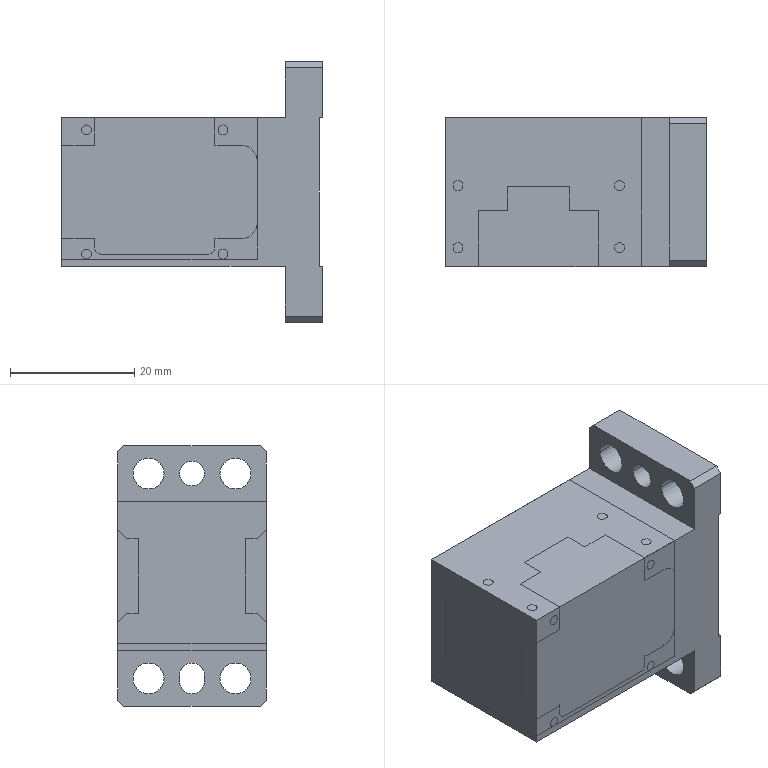NC program | NX | posted with a generic post | part box 42 x 24 x 42 mm
Lines 10409 to 10692 of 10692:
(PLANAR_MILL_COPY_2 , TOOL : D6A45)
N20798 T07 M6
N20800 G54
N20802 G17 G0 G90 X-6.753 Y16.814 B0. C0. S7500 M3
N20804 G43 Z30. H7
N20806 Z0.5
N20808 G94 G1 Z-1. F1250.
N20810 X-6.134 Y17.6
N20812 G3 X-7. Y18.1 R1.
N20814 X-8.6 Y16.5 R1.6
N20816 X-7. Y18.1 R-1.6
N20818 X-7.866 Y17.6 R1.
N20820 G1 X-7.247 Y16.814
N20822 Z0.5
N20824 G0 Z30.
N20826 X-1.063 Y16.825
N20828 Z0.5
N20830 G1 X-1.1 Y16.759 Z0.48
N20832 Y16.5 Z0.41
N20834 Y16.241 Z0.341
N20836 X-0.799 Y15.701 Z0.175
N20838 X-0.259 Y15.4 Z0.009
N20840 X0.259 Z-0.129
N20842 X0.799 Y15.701 Z-0.295
N20844 X1.1 Y16.241 Z-0.461
N20846 Y16.759 Z-0.599
N20848 X0.799 Y17.299 Z-0.765
N20850 X0.259 Y17.6 Z-0.931
N20852 X0. Z-1.
N20854 G3 X-1.1 Y16.5 R1.1
N20856 X0. Y17.6 R-1.1
N20858 X-0.866 Y17.1 R1.
N20860 G1 Z0.5
N20862 G0 Z30.
N20864 X7.247 Y16.814
N20866 Z0.5
N20868 G1 Z-1.
N20870 X7.866 Y17.6
N20872 G3 X7. Y18.1 R1.
N20874 X5.4 Y16.5 R1.6
N20876 X7. Y18.1 R-1.6
N20878 X6.134 Y17.6 R1.
N20880 G1 X6.753 Y16.814
N20882 Z0.5
N20884 G0 Z30.
N20886 X-14.345 Y12.711
N20888 Z0.5
N20890 G1 Z-1.
N20892 X-13.861 Y12.591
N20894 G3 X-12.9 Y12.867 R1.
N20896 G1 Y19.959
N20898 G2 X-12.607 Y20.666 R1.
N20900 G1 X-11.666 Y21.607
N20902 G2 X-10.959 Y21.9 R1.
N20904 G1 X10.959
N20906 G2 X11.666 Y21.607 R1.
N20908 G1 X12.607 Y20.666
N20910 G2 X12.9 Y19.959 R1.
N20912 G1 Y12.867
N20914 G3 X13.861 Y12.591 R1.
N20916 G1 X14.345 Y12.711
N20918 Z0.5
N20920 G0 Z30.
N20922 Y-12.711
N20924 Z0.5
N20926 G1 Z-1.
N20928 X13.861 Y-12.591
N20930 G3 X12.9 Y-12.867 R1.
N20932 G1 Y-19.959
N20934 G2 X12.607 Y-20.666 R1.
N20936 G1 X11.666 Y-21.607
N20938 G2 X10.959 Y-21.9 R1.
N20940 G1 X-10.959
N20942 G2 X-11.666 Y-21.607 R1.
N20944 G1 X-12.607 Y-20.666
N20946 G2 X-12.9 Y-19.959 R1.
N20948 G1 Y-12.867
N20950 G3 X-13.861 Y-12.591 R1.
N20952 G1 X-14.345 Y-12.711
N20954 Z0.5
N20956 G0 Z30.
N20958 X-7.247 Y-16.814
N20960 Z0.5
N20962 G1 Z-1.
N20964 X-7.866 Y-17.6
N20966 G3 X-7. Y-18.1 R1.
N20968 X-5.4 Y-16.5 R1.6
N20970 X-7. Y-18.1 R-1.6
N20972 X-6.134 Y-17.6 R1.
N20974 G1 X-6.753 Y-16.814
N20976 Z0.5
N20978 G0 Z30.
N20980 X-0.939 Y-15.452
N20982 Z0.5
N20984 G1 X-1.1 Y-15.741 Z0.411
N20986 Y-17.259 Z0.005
N20988 X-0.799 Y-17.799 Z-0.161
N20990 X-0.259 Y-18.1 Z-0.327
N20992 X0.259 Z-0.465
N20994 X0.799 Y-17.799 Z-0.631
N20996 X1.1 Y-17.259 Z-0.797
N20998 Y-16.5 Z-1.
N21000 Y-16.
N21002 G3 X0. Y-14.9 R1.1
N21004 X-1.1 Y-16. R1.1
N21006 G1 Y-17.
N21008 G3 X0. Y-18.1 R1.1
N21010 X1.1 Y-17. R1.1
N21012 G1 Y-16.5
N21014 G3 X0.6 Y-15.634 R1.
N21016 G1 Z0.5
N21018 G0 Z30.
N21020 X6.753 Y-16.814
N21022 Z0.5
N21024 G1 Z-1.
N21026 X6.134 Y-17.6
N21028 G3 X7. Y-18.1 R1.
N21030 X8.6 Y-16.5 R1.6
N21032 X7. Y-18.1 R-1.6
N21034 X7.866 Y-17.6 R1.
N21036 G1 X7.247 Y-16.814
N21038 Z0.5
N21040 G0 Z30.
(PLANAR_MILL_COPY_2_COPY , TOOL : D6A45)
N21042 X-14.369 Y-9.849
N21044 Z0.
N21046 G1 Z-1.5
N21048 X-13.898 Y-10.157
N21050 G3 X-12.9 Y-10.214 R1.
N21052 G1 Y10.214
N21054 G3 X-13.898 Y10.157 R1.
N21056 G1 X-14.369 Y9.849
N21058 Z0.
N21060 G0 Z30.
N21062 X14.369
N21064 Z0.
N21066 G1 Z-1.5
N21068 X13.898 Y10.157
N21070 G3 X12.9 Y10.214 R1.
N21072 G1 Y-10.214
N21074 G3 X13.898 Y-10.157 R1.
N21076 G1 X14.369 Y-9.849
N21078 Z0.
N21080 G0 Z30.
N21082 M5
(刀补 , TOOL : D3)
N21084 T03 M6
N21086 G54
N21088 G17 G0 G90 X-0.056 Y-16.163 B0. C0. S6500 M3
N21090 G43 Z30. H3
N21092 Z-1.
N21094 G94 G1 Z-2. F1000.
N21096 G41 X-0.15 Y-16.197 D3
N21098 X-0.3 Y-16.284
N21100 G3 X-0.45 Y-16.544 R0.3
N21102 G1 Y-17.
N21104 G3 X0. Y-17.45 R0.45
N21106 X0.45 Y-17. R0.45
N21108 G1 Y-16.
N21110 G3 X0. Y-15.55 R0.45
N21112 X-0.45 Y-16. R0.45
N21114 G1 Y-16.544
N21116 Y-16.785 Z-2.133
N21118 Y-16.906 Z-2.2
N21120 X-0.449 Y-17.026 Z-2.267
N21122 X-0.432 Y-17.126 Z-2.322
N21124 X-0.416 Y-17.172 Z-2.349
N21126 X-0.403 Y-17.2 Z-2.366
N21128 X-0.373 Y-17.252 Z-2.4
N21130 X-0.308 Y-17.328 Z-2.454
N21132 X-0.271 Y-17.359 Z-2.481
N21134 X-0.246 Y-17.377 Z-2.498
N21136 X-0.192 Y-17.407 Z-2.533
N21138 X-0.098 Y-17.439 Z-2.587
N21140 X-0.05 Y-17.447 Z-2.614
N21142 X-0.019 Y-17.45 Z-2.632
N21144 X0.043 Y-17.448 Z-2.667
N21146 X0.141 Y-17.428 Z-2.721
N21148 X0.186 Y-17.41 Z-2.748
N21150 X0.213 Y-17.396 Z-2.765
N21152 X0.266 Y-17.363 Z-2.8
N21154 X0.338 Y-17.297 Z-2.853
N21156 X0.368 Y-17.259 Z-2.88
N21158 X0.385 Y-17.233 Z-2.898
N21160 X0.414 Y-17.176 Z-2.933
N21162 X0.432 Y-17.128 Z-2.962
N21164 X0.438 Y-17.103 Z-2.976
N21166 X0.447 Y-17.05 Z-3.006
N21168 X0.45 Y-16.939 Z-3.067
N21170 Y-16.215 Z-3.467
N21172 Y-16.094 Z-3.533
N21174 X0.449 Y-15.974 Z-3.6
N21176 X0.432 Y-15.874 Z-3.655
N21178 X0.416 Y-15.828 Z-3.683
N21180 X0.403 Y-15.8 Z-3.699
N21182 X0.373 Y-15.748 Z-3.733
N21184 X0.308 Y-15.672 Z-3.787
N21186 X0.271 Y-15.641 Z-3.814
N21188 X0.246 Y-15.623 Z-3.832
N21190 X0.192 Y-15.593 Z-3.867
N21192 X0.135 Y-15.571 Z-3.9
N21194 X0.077 Y-15.557 Z-3.933
N21196 X0.017 Y-15.55 Z-3.967
N21198 X-0.043 Y-15.552 Z-4.
N21200 G3 X-0.45 Y-16. R0.45
N21202 G1 Y-16.544
N21204 Y-16.785 Z-4.133
N21206 Y-16.906 Z-4.2
N21208 X-0.449 Y-17.026 Z-4.267
N21210 X-0.432 Y-17.126 Z-4.322
N21212 X-0.416 Y-17.172 Z-4.349
N21214 X-0.403 Y-17.2 Z-4.366
N21216 X-0.373 Y-17.252 Z-4.4
N21218 X-0.308 Y-17.328 Z-4.454
N21220 X-0.271 Y-17.359 Z-4.481
N21222 X-0.246 Y-17.377 Z-4.498
N21224 X-0.192 Y-17.407 Z-4.533
N21226 X-0.098 Y-17.439 Z-4.587
N21228 X-0.05 Y-17.447 Z-4.614
N21230 X-0.019 Y-17.45 Z-4.632
N21232 X0.043 Y-17.448 Z-4.667
N21234 X0.141 Y-17.428 Z-4.721
N21236 X0.186 Y-17.41 Z-4.748
N21238 X0.213 Y-17.396 Z-4.765
N21240 X0.266 Y-17.363 Z-4.8
N21242 X0.338 Y-17.297 Z-4.853
N21244 X0.368 Y-17.259 Z-4.88
N21246 X0.385 Y-17.233 Z-4.898
N21248 X0.414 Y-17.176 Z-4.933
N21250 X0.432 Y-17.128 Z-4.962
N21252 X0.438 Y-17.103 Z-4.976
N21254 X0.447 Y-17.05 Z-5.006
N21256 X0.45 Y-16.939 Z-5.067
N21258 Y-16.215 Z-5.467
N21260 Y-16.094 Z-5.533
N21262 X0.449 Y-15.974 Z-5.6
N21264 X0.432 Y-15.874 Z-5.655
N21266 X0.416 Y-15.828 Z-5.683
N21268 X0.403 Y-15.8 Z-5.699
N21270 X0.373 Y-15.748 Z-5.733
N21272 X0.308 Y-15.672 Z-5.787
N21274 X0.271 Y-15.641 Z-5.814
N21276 X0.246 Y-15.623 Z-5.832
N21278 X0.192 Y-15.593 Z-5.867
N21280 X0.135 Y-15.571 Z-5.9
N21282 X0.077 Y-15.557 Z-5.933
N21284 X0.017 Y-15.55 Z-5.967
N21286 X-0.043 Y-15.552 Z-6.
N21288 G3 X-0.45 Y-16. R0.45
N21290 G1 Y-17.
N21292 G3 X0. Y-17.45 R0.45
N21294 X0.45 Y-17. R0.45
N21296 G1 Y-16.
N21298 G3 X-0.043 Y-15.552 R0.45
N21300 X-0.288 Y-15.727 R0.3
N21302 G40
N21304 G1 X-0.109 Y-15.897
N21306 Z-5.
N21308 G0 Z30.
(刀补3 , TOOL : D3)
N21310 X0. Y16.5
N21312 Z0.5
N21314 G41 G1 X0.027 Y16.404
N21316 G3 X0.45 Y16.5 R0.222
N21318 X0.45 Y16.5 Z-1.5 I-0.45 J0.
N21320 X0.45 Y16.5 Z-3.5 I-0.45 J0.
N21322 X0.45 Y16.5 Z-5.5 I-0.45 J0.
N21324 X0. Y16.95 Z-6. R0.45
N21326 X-0.45 Y16.5 R0.45
N21328 X0. Y16.95 R-0.45
N21330 X-0.096 Y16.527 R0.222
N21332 G40
N21334 G1 X0. Y16.5
N21336 G0 Z30.
N21338 M5
N21340 M2